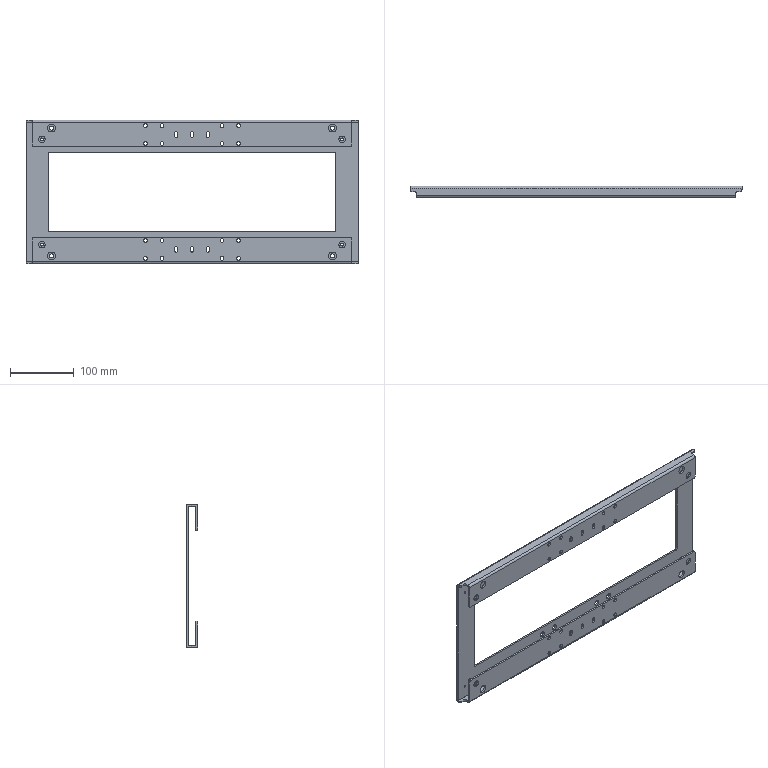Part | SolidWorks | features BaseBody 1 | 1 solid | 220 faces | box 520 x 17.8 x 225 mm | volume 330533 mm3 | cylinder 166 | plane 54 | commonest cylinder face diameters 6 x48 9 x44 5 x18 2.5 x16 4.2 x8 6.5 x8